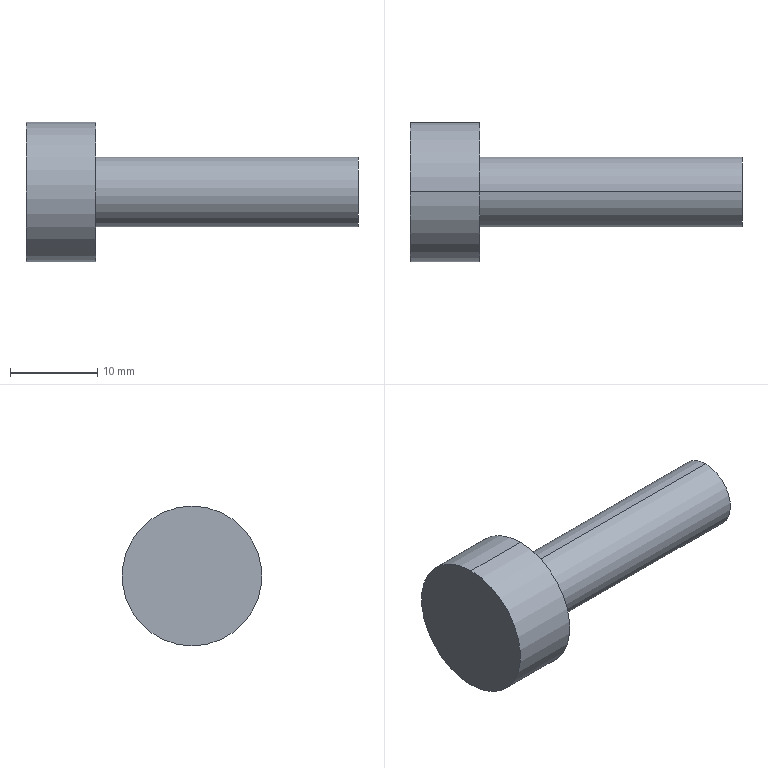Part | STEP file | 1 solid | 7 faces | box 38 x 16 x 16 mm | volume 3116 mm3 | cylinder 4 | plane 3 | commonest cylinder face diameters 8 x2 16 x2
STEP:
#1=CARTESIAN_POINT('',(0.,0.,0.));
#2=DIRECTION('',(0.,0.,1.));
#3=DIRECTION('',(1.,0.,0.));
#4=AXIS2_PLACEMENT_3D('',#1,#2,#3);
#5=CARTESIAN_POINT('',(-38.,0.,-8.));
#6=VERTEX_POINT('',#5);
#7=CARTESIAN_POINT('',(-38.,0.,8.));
#8=VERTEX_POINT('',#7);
#9=CARTESIAN_POINT('',(-38.,0.,0.));
#10=DIRECTION('',(1.,0.,0.));
#11=DIRECTION('',(0.,0.,-1.));
#12=AXIS2_PLACEMENT_3D('',#9,#10,#11);
#13=CIRCLE('',#12,8.);
#14=CARTESIAN_POINT('',(0.,0.,0.));
#15=DIRECTION('',(1.,0.,0.));
#16=DIRECTION('',(0.,0.,-1.));
#17=AXIS2_PLACEMENT_3D('',#14,#15,#16);
#18=CYLINDRICAL_SURFACE('',#17,8.);
#19=CARTESIAN_POINT('',(0.,-38.));
#20=DIRECTION('',(1.,0.));
#21=VECTOR('',#20,1.);
#22=LINE('',#19,#21);
#23=(GEOMETRIC_REPRESENTATION_CONTEXT(2)PARAMETRIC_REPRESENTATION_CONTEXT()REPRESENTATION_CONTEXT('',''));
#24=DEFINITIONAL_REPRESENTATION('',(#22),#23);
#25=PCURVE('',#18,#24);
#26=CARTESIAN_POINT('',(-38.,8.,0.));
#27=DIRECTION('',(-1.,0.,0.));
#28=DIRECTION('',(0.,0.,1.));
#29=AXIS2_PLACEMENT_3D('',#26,#27,#28);
#30=PLANE('',#29);
#31=CARTESIAN_POINT('',(-8.,-8.));
#32=CARTESIAN_POINT('',(-8.,5.856));
#33=CARTESIAN_POINT('',(4.,-1.072));
#34=CARTESIAN_POINT('',(16.,-8.));
#35=CARTESIAN_POINT('',(4.,-14.928));
#36=CARTESIAN_POINT('',(-8.,-21.856));
#37=CARTESIAN_POINT('',(-8.,-8.));
#38=(BOUNDED_CURVE()B_SPLINE_CURVE(2,(#31,#32,#33,#34,#35,#36,#37),.UNSPECIFIED.,.T.,.F.)B_SPLINE_CURVE_WITH_KNOTS((1,2,2,2,2,1),(-2.094,0.,2.094,4.189,6.283,8.378),.UNSPECIFIED.)CURVE()GEOMETRIC_REPRESENTATION_ITEM()RATIONAL_B_SPLINE_CURVE((1.,0.5,1.,0.5,1.,0.5,1.))REPRESENTATION_ITEM(''));
#39=(GEOMETRIC_REPRESENTATION_CONTEXT(2)PARAMETRIC_REPRESENTATION_CONTEXT()REPRESENTATION_CONTEXT('',''));
#40=DEFINITIONAL_REPRESENTATION('',(#38),#39);
#41=PCURVE('',#30,#40);
#42=SURFACE_CURVE('',#13,(#25,#41),.PCURVE_S1.);
#43=EDGE_CURVE('',#6,#8,#42,.T.);
#44=ORIENTED_EDGE('',*,*,#43,.T.);
#45=CARTESIAN_POINT('',(-30.,0.,8.));
#46=VERTEX_POINT('',#45);
#47=CARTESIAN_POINT('',(0.,0.,8.));
#48=DIRECTION('',(1.,0.,0.));
#49=VECTOR('',#48,1.);
#50=LINE('',#47,#49);
#51=CARTESIAN_POINT('',(3.142,0.));
#52=DIRECTION('',(0.,1.));
#53=VECTOR('',#52,1.);
#54=LINE('',#51,#53);
#55=(GEOMETRIC_REPRESENTATION_CONTEXT(2)PARAMETRIC_REPRESENTATION_CONTEXT()REPRESENTATION_CONTEXT('',''));
#56=DEFINITIONAL_REPRESENTATION('',(#54),#55);
#57=PCURVE('',#18,#56);
#58=CARTESIAN_POINT('',(0.,0.,0.));
#59=DIRECTION('',(1.,0.,0.));
#60=DIRECTION('',(0.,0.,-1.));
#61=AXIS2_PLACEMENT_3D('',#58,#59,#60);
#62=CYLINDRICAL_SURFACE('',#61,8.);
#63=CARTESIAN_POINT('',(3.142,0.));
#64=DIRECTION('',(0.,1.));
#65=VECTOR('',#64,1.);
#66=LINE('',#63,#65);
#67=(GEOMETRIC_REPRESENTATION_CONTEXT(2)PARAMETRIC_REPRESENTATION_CONTEXT()REPRESENTATION_CONTEXT('',''));
#68=DEFINITIONAL_REPRESENTATION('',(#66),#67);
#69=PCURVE('',#62,#68);
#70=SURFACE_CURVE('',#50,(#57,#69),.PCURVE_S1.);
#71=EDGE_CURVE('',#8,#46,#70,.T.);
#72=ORIENTED_EDGE('',*,*,#71,.T.);
#73=CARTESIAN_POINT('',(-30.,0.,-8.));
#74=VERTEX_POINT('',#73);
#75=CARTESIAN_POINT('',(-30.,0.,0.));
#76=DIRECTION('',(1.,0.,0.));
#77=DIRECTION('',(0.,0.,-1.));
#78=AXIS2_PLACEMENT_3D('',#75,#76,#77);
#79=CIRCLE('',#78,8.);
#80=CARTESIAN_POINT('',(0.,-30.));
#81=DIRECTION('',(1.,0.));
#82=VECTOR('',#81,1.);
#83=LINE('',#80,#82);
#84=(GEOMETRIC_REPRESENTATION_CONTEXT(2)PARAMETRIC_REPRESENTATION_CONTEXT()REPRESENTATION_CONTEXT('',''));
#85=DEFINITIONAL_REPRESENTATION('',(#83),#84);
#86=PCURVE('',#18,#85);
#87=CARTESIAN_POINT('',(-30.,4.,0.));
#88=DIRECTION('',(1.,0.,0.));
#89=DIRECTION('',(0.,0.,-1.));
#90=AXIS2_PLACEMENT_3D('',#87,#88,#89);
#91=PLANE('',#90);
#92=CARTESIAN_POINT('',(0.,-4.));
#93=DIRECTION('',(1.,0.));
#94=AXIS2_PLACEMENT_2D('',#92,#93);
#95=CIRCLE('',#94,8.);
#96=(GEOMETRIC_REPRESENTATION_CONTEXT(2)PARAMETRIC_REPRESENTATION_CONTEXT()REPRESENTATION_CONTEXT('',''));
#97=DEFINITIONAL_REPRESENTATION('',(#95),#96);
#98=PCURVE('',#91,#97);
#99=SURFACE_CURVE('',#79,(#86,#98),.PCURVE_S1.);
#100=EDGE_CURVE('',#74,#46,#99,.T.);
#101=ORIENTED_EDGE('',*,*,#100,.F.);
#102=CARTESIAN_POINT('',(0.,0.,-8.));
#103=DIRECTION('',(1.,0.,0.));
#104=VECTOR('',#103,1.);
#105=LINE('',#102,#104);
#106=CARTESIAN_POINT('',(0.,0.));
#107=DIRECTION('',(0.,1.));
#108=VECTOR('',#107,1.);
#109=LINE('',#106,#108);
#110=(GEOMETRIC_REPRESENTATION_CONTEXT(2)PARAMETRIC_REPRESENTATION_CONTEXT()REPRESENTATION_CONTEXT('',''));
#111=DEFINITIONAL_REPRESENTATION('',(#109),#110);
#112=PCURVE('',#18,#111);
#113=CARTESIAN_POINT('',(6.283,0.));
#114=DIRECTION('',(0.,1.));
#115=VECTOR('',#114,1.);
#116=LINE('',#113,#115);
#117=(GEOMETRIC_REPRESENTATION_CONTEXT(2)PARAMETRIC_REPRESENTATION_CONTEXT()REPRESENTATION_CONTEXT('',''));
#118=DEFINITIONAL_REPRESENTATION('',(#116),#117);
#119=PCURVE('',#62,#118);
#120=SURFACE_CURVE('',#105,(#112,#119),.PCURVE_S1.);
#121=EDGE_CURVE('',#6,#74,#120,.T.);
#122=ORIENTED_EDGE('',*,*,#121,.F.);
#123=EDGE_LOOP('',(#44,#72,#101,#122));
#124=FACE_BOUND('',#123,.T.);
#125=ADVANCED_FACE('',(#124),#18,.T.);
#126=CARTESIAN_POINT('',(-30.,0.,-4.));
#127=VERTEX_POINT('',#126);
#128=CARTESIAN_POINT('',(-30.,0.,4.));
#129=VERTEX_POINT('',#128);
#130=CARTESIAN_POINT('',(-30.,0.,0.));
#131=DIRECTION('',(1.,0.,0.));
#132=DIRECTION('',(0.,0.,-1.));
#133=AXIS2_PLACEMENT_3D('',#130,#131,#132);
#134=CIRCLE('',#133,4.);
#135=CARTESIAN_POINT('',(0.,0.,0.));
#136=DIRECTION('',(1.,0.,0.));
#137=DIRECTION('',(0.,0.,-1.));
#138=AXIS2_PLACEMENT_3D('',#135,#136,#137);
#139=CYLINDRICAL_SURFACE('',#138,4.);
#140=CARTESIAN_POINT('',(0.,-30.));
#141=DIRECTION('',(1.,0.));
#142=VECTOR('',#141,1.);
#143=LINE('',#140,#142);
#144=(GEOMETRIC_REPRESENTATION_CONTEXT(2)PARAMETRIC_REPRESENTATION_CONTEXT()REPRESENTATION_CONTEXT('',''));
#145=DEFINITIONAL_REPRESENTATION('',(#143),#144);
#146=PCURVE('',#139,#145);
#147=CARTESIAN_POINT('',(0.,-4.));
#148=DIRECTION('',(1.,0.));
#149=AXIS2_PLACEMENT_2D('',#147,#148);
#150=CIRCLE('',#149,4.);
#151=(GEOMETRIC_REPRESENTATION_CONTEXT(2)PARAMETRIC_REPRESENTATION_CONTEXT()REPRESENTATION_CONTEXT('',''));
#152=DEFINITIONAL_REPRESENTATION('',(#150),#151);
#153=PCURVE('',#91,#152);
#154=SURFACE_CURVE('',#134,(#146,#153),.PCURVE_S1.);
#155=EDGE_CURVE('',#127,#129,#154,.T.);
#156=ORIENTED_EDGE('',*,*,#155,.T.);
#157=CARTESIAN_POINT('',(0.,0.,4.));
#158=VERTEX_POINT('',#157);
#159=CARTESIAN_POINT('',(0.,0.,4.));
#160=DIRECTION('',(1.,0.,0.));
#161=VECTOR('',#160,1.);
#162=LINE('',#159,#161);
#163=CARTESIAN_POINT('',(3.142,0.));
#164=DIRECTION('',(0.,1.));
#165=VECTOR('',#164,1.);
#166=LINE('',#163,#165);
#167=(GEOMETRIC_REPRESENTATION_CONTEXT(2)PARAMETRIC_REPRESENTATION_CONTEXT()REPRESENTATION_CONTEXT('',''));
#168=DEFINITIONAL_REPRESENTATION('',(#166),#167);
#169=PCURVE('',#139,#168);
#170=CARTESIAN_POINT('',(0.,0.,0.));
#171=DIRECTION('',(1.,0.,0.));
#172=DIRECTION('',(0.,0.,-1.));
#173=AXIS2_PLACEMENT_3D('',#170,#171,#172);
#174=CYLINDRICAL_SURFACE('',#173,4.);
#175=CARTESIAN_POINT('',(3.142,0.));
#176=DIRECTION('',(0.,1.));
#177=VECTOR('',#176,1.);
#178=LINE('',#175,#177);
#179=(GEOMETRIC_REPRESENTATION_CONTEXT(2)PARAMETRIC_REPRESENTATION_CONTEXT()REPRESENTATION_CONTEXT('',''));
#180=DEFINITIONAL_REPRESENTATION('',(#178),#179);
#181=PCURVE('',#174,#180);
#182=SURFACE_CURVE('',#162,(#169,#181),.PCURVE_S1.);
#183=EDGE_CURVE('',#129,#158,#182,.T.);
#184=ORIENTED_EDGE('',*,*,#183,.T.);
#185=CARTESIAN_POINT('',(0.,0.,-4.));
#186=VERTEX_POINT('',#185);
#187=CARTESIAN_POINT('',(0.,0.,0.));
#188=DIRECTION('',(1.,0.,0.));
#189=DIRECTION('',(0.,0.,-1.));
#190=AXIS2_PLACEMENT_3D('',#187,#188,#189);
#191=CIRCLE('',#190,4.);
#192=CARTESIAN_POINT('',(0.,0.));
#193=DIRECTION('',(1.,0.));
#194=VECTOR('',#193,1.);
#195=LINE('',#192,#194);
#196=(GEOMETRIC_REPRESENTATION_CONTEXT(2)PARAMETRIC_REPRESENTATION_CONTEXT()REPRESENTATION_CONTEXT('',''));
#197=DEFINITIONAL_REPRESENTATION('',(#195),#196);
#198=PCURVE('',#139,#197);
#199=CARTESIAN_POINT('',(0.,0.,0.));
#200=DIRECTION('',(1.,0.,0.));
#201=DIRECTION('',(0.,0.,-1.));
#202=AXIS2_PLACEMENT_3D('',#199,#200,#201);
#203=PLANE('',#202);
#204=CARTESIAN_POINT('',(0.,0.));
#205=DIRECTION('',(1.,0.));
#206=AXIS2_PLACEMENT_2D('',#204,#205);
#207=CIRCLE('',#206,4.);
#208=(GEOMETRIC_REPRESENTATION_CONTEXT(2)PARAMETRIC_REPRESENTATION_CONTEXT()REPRESENTATION_CONTEXT('',''));
#209=DEFINITIONAL_REPRESENTATION('',(#207),#208);
#210=PCURVE('',#203,#209);
#211=SURFACE_CURVE('',#191,(#198,#210),.PCURVE_S1.);
#212=EDGE_CURVE('',#186,#158,#211,.T.);
#213=ORIENTED_EDGE('',*,*,#212,.F.);
#214=CARTESIAN_POINT('',(0.,0.,-4.));
#215=DIRECTION('',(1.,0.,0.));
#216=VECTOR('',#215,1.);
#217=LINE('',#214,#216);
#218=CARTESIAN_POINT('',(0.,0.));
#219=DIRECTION('',(0.,1.));
#220=VECTOR('',#219,1.);
#221=LINE('',#218,#220);
#222=(GEOMETRIC_REPRESENTATION_CONTEXT(2)PARAMETRIC_REPRESENTATION_CONTEXT()REPRESENTATION_CONTEXT('',''));
#223=DEFINITIONAL_REPRESENTATION('',(#221),#222);
#224=PCURVE('',#139,#223);
#225=CARTESIAN_POINT('',(6.283,0.));
#226=DIRECTION('',(0.,1.));
#227=VECTOR('',#226,1.);
#228=LINE('',#225,#227);
#229=(GEOMETRIC_REPRESENTATION_CONTEXT(2)PARAMETRIC_REPRESENTATION_CONTEXT()REPRESENTATION_CONTEXT('',''));
#230=DEFINITIONAL_REPRESENTATION('',(#228),#229);
#231=PCURVE('',#174,#230);
#232=SURFACE_CURVE('',#217,(#224,#231),.PCURVE_S1.);
#233=EDGE_CURVE('',#127,#186,#232,.T.);
#234=ORIENTED_EDGE('',*,*,#233,.F.);
#235=EDGE_LOOP('',(#156,#184,#213,#234));
#236=FACE_BOUND('',#235,.T.);
#237=ADVANCED_FACE('',(#236),#139,.T.);
#238=ORIENTED_EDGE('',*,*,#212,.T.);
#239=CARTESIAN_POINT('',(0.,0.,0.));
#240=DIRECTION('',(1.,0.,0.));
#241=DIRECTION('',(0.,0.,-1.));
#242=AXIS2_PLACEMENT_3D('',#239,#240,#241);
#243=CIRCLE('',#242,4.);
#244=CARTESIAN_POINT('',(0.,0.));
#245=DIRECTION('',(1.,0.));
#246=AXIS2_PLACEMENT_2D('',#244,#245);
#247=CIRCLE('',#246,4.);
#248=(GEOMETRIC_REPRESENTATION_CONTEXT(2)PARAMETRIC_REPRESENTATION_CONTEXT()REPRESENTATION_CONTEXT('',''));
#249=DEFINITIONAL_REPRESENTATION('',(#247),#248);
#250=PCURVE('',#203,#249);
#251=CARTESIAN_POINT('',(0.,0.));
#252=DIRECTION('',(1.,0.));
#253=VECTOR('',#252,1.);
#254=LINE('',#251,#253);
#255=(GEOMETRIC_REPRESENTATION_CONTEXT(2)PARAMETRIC_REPRESENTATION_CONTEXT()REPRESENTATION_CONTEXT('',''));
#256=DEFINITIONAL_REPRESENTATION('',(#254),#255);
#257=PCURVE('',#174,#256);
#258=SURFACE_CURVE('',#243,(#250,#257),.PCURVE_S1.);
#259=EDGE_CURVE('',#158,#186,#258,.T.);
#260=ORIENTED_EDGE('',*,*,#259,.T.);
#261=EDGE_LOOP('',(#238,#260));
#262=FACE_BOUND('',#261,.T.);
#263=ADVANCED_FACE('',(#262),#203,.T.);
#264=ORIENTED_EDGE('',*,*,#183,.F.);
#265=CARTESIAN_POINT('',(-30.,0.,0.));
#266=DIRECTION('',(1.,0.,0.));
#267=DIRECTION('',(0.,0.,-1.));
#268=AXIS2_PLACEMENT_3D('',#265,#266,#267);
#269=CIRCLE('',#268,4.);
#270=CARTESIAN_POINT('',(0.,-30.));
#271=DIRECTION('',(1.,0.));
#272=VECTOR('',#271,1.);
#273=LINE('',#270,#272);
#274=(GEOMETRIC_REPRESENTATION_CONTEXT(2)PARAMETRIC_REPRESENTATION_CONTEXT()REPRESENTATION_CONTEXT('',''));
#275=DEFINITIONAL_REPRESENTATION('',(#273),#274);
#276=PCURVE('',#174,#275);
#277=CARTESIAN_POINT('',(0.,-4.));
#278=DIRECTION('',(1.,0.));
#279=AXIS2_PLACEMENT_2D('',#277,#278);
#280=CIRCLE('',#279,4.);
#281=(GEOMETRIC_REPRESENTATION_CONTEXT(2)PARAMETRIC_REPRESENTATION_CONTEXT()REPRESENTATION_CONTEXT('',''));
#282=DEFINITIONAL_REPRESENTATION('',(#280),#281);
#283=PCURVE('',#91,#282);
#284=SURFACE_CURVE('',#269,(#276,#283),.PCURVE_S1.);
#285=EDGE_CURVE('',#129,#127,#284,.T.);
#286=ORIENTED_EDGE('',*,*,#285,.T.);
#287=ORIENTED_EDGE('',*,*,#233,.T.);
#288=ORIENTED_EDGE('',*,*,#259,.F.);
#289=EDGE_LOOP('',(#264,#286,#287,#288));
#290=FACE_BOUND('',#289,.T.);
#291=ADVANCED_FACE('',(#290),#174,.T.);
#292=ORIENTED_EDGE('',*,*,#100,.T.);
#293=CARTESIAN_POINT('',(-30.,0.,0.));
#294=DIRECTION('',(1.,0.,0.));
#295=DIRECTION('',(0.,0.,-1.));
#296=AXIS2_PLACEMENT_3D('',#293,#294,#295);
#297=CIRCLE('',#296,8.);
#298=CARTESIAN_POINT('',(0.,-4.));
#299=DIRECTION('',(1.,0.));
#300=AXIS2_PLACEMENT_2D('',#298,#299);
#301=CIRCLE('',#300,8.);
#302=(GEOMETRIC_REPRESENTATION_CONTEXT(2)PARAMETRIC_REPRESENTATION_CONTEXT()REPRESENTATION_CONTEXT('',''));
#303=DEFINITIONAL_REPRESENTATION('',(#301),#302);
#304=PCURVE('',#91,#303);
#305=CARTESIAN_POINT('',(0.,-30.));
#306=DIRECTION('',(1.,0.));
#307=VECTOR('',#306,1.);
#308=LINE('',#305,#307);
#309=(GEOMETRIC_REPRESENTATION_CONTEXT(2)PARAMETRIC_REPRESENTATION_CONTEXT()REPRESENTATION_CONTEXT('',''));
#310=DEFINITIONAL_REPRESENTATION('',(#308),#309);
#311=PCURVE('',#62,#310);
#312=SURFACE_CURVE('',#297,(#304,#311),.PCURVE_S1.);
#313=EDGE_CURVE('',#46,#74,#312,.T.);
#314=ORIENTED_EDGE('',*,*,#313,.T.);
#315=EDGE_LOOP('',(#292,#314));
#316=FACE_BOUND('',#315,.T.);
#317=ORIENTED_EDGE('',*,*,#155,.F.);
#318=ORIENTED_EDGE('',*,*,#285,.F.);
#319=EDGE_LOOP('',(#317,#318));
#320=FACE_BOUND('',#319,.T.);
#321=ADVANCED_FACE('',(#316,#320),#91,.T.);
#322=ORIENTED_EDGE('',*,*,#71,.F.);
#323=CARTESIAN_POINT('',(-38.,0.,0.));
#324=DIRECTION('',(1.,0.,0.));
#325=DIRECTION('',(0.,0.,-1.));
#326=AXIS2_PLACEMENT_3D('',#323,#324,#325);
#327=CIRCLE('',#326,8.);
#328=CARTESIAN_POINT('',(0.,-38.));
#329=DIRECTION('',(1.,0.));
#330=VECTOR('',#329,1.);
#331=LINE('',#328,#330);
#332=(GEOMETRIC_REPRESENTATION_CONTEXT(2)PARAMETRIC_REPRESENTATION_CONTEXT()REPRESENTATION_CONTEXT('',''));
#333=DEFINITIONAL_REPRESENTATION('',(#331),#332);
#334=PCURVE('',#62,#333);
#335=CARTESIAN_POINT('',(-8.,-8.));
#336=CARTESIAN_POINT('',(-8.,5.856));
#337=CARTESIAN_POINT('',(4.,-1.072));
#338=CARTESIAN_POINT('',(16.,-8.));
#339=CARTESIAN_POINT('',(4.,-14.928));
#340=CARTESIAN_POINT('',(-8.,-21.856));
#341=CARTESIAN_POINT('',(-8.,-8.));
#342=(BOUNDED_CURVE()B_SPLINE_CURVE(2,(#335,#336,#337,#338,#339,#340,#341),.UNSPECIFIED.,.T.,.F.)B_SPLINE_CURVE_WITH_KNOTS((1,2,2,2,2,1),(-2.094,0.,2.094,4.189,6.283,8.378),.UNSPECIFIED.)CURVE()GEOMETRIC_REPRESENTATION_ITEM()RATIONAL_B_SPLINE_CURVE((1.,0.5,1.,0.5,1.,0.5,1.))REPRESENTATION_ITEM(''));
#343=(GEOMETRIC_REPRESENTATION_CONTEXT(2)PARAMETRIC_REPRESENTATION_CONTEXT()REPRESENTATION_CONTEXT('',''));
#344=DEFINITIONAL_REPRESENTATION('',(#342),#343);
#345=PCURVE('',#30,#344);
#346=SURFACE_CURVE('',#327,(#334,#345),.PCURVE_S1.);
#347=EDGE_CURVE('',#8,#6,#346,.T.);
#348=ORIENTED_EDGE('',*,*,#347,.T.);
#349=ORIENTED_EDGE('',*,*,#121,.T.);
#350=ORIENTED_EDGE('',*,*,#313,.F.);
#351=EDGE_LOOP('',(#322,#348,#349,#350));
#352=FACE_BOUND('',#351,.T.);
#353=ADVANCED_FACE('',(#352),#62,.T.);
#354=ORIENTED_EDGE('',*,*,#43,.F.);
#355=ORIENTED_EDGE('',*,*,#347,.F.);
#356=EDGE_LOOP('',(#354,#355));
#357=FACE_BOUND('',#356,.T.);
#358=ADVANCED_FACE('',(#357),#30,.T.);
#359=CLOSED_SHELL('',(#125,#237,#263,#291,#321,#353,#358));
#360=MANIFOLD_SOLID_BREP('',#359);
#361=(LENGTH_UNIT()NAMED_UNIT(*)SI_UNIT(.MILLI.,.METRE.));
#362=UNCERTAINTY_MEASURE_WITH_UNIT(LENGTH_MEASURE(0.0000001),#361,'','');
#363=(NAMED_UNIT(*)PLANE_ANGLE_UNIT()SI_UNIT($,.RADIAN.));
#364=(NAMED_UNIT(*)SI_UNIT($,.STERADIAN.)SOLID_ANGLE_UNIT());
#365=(GEOMETRIC_REPRESENTATION_CONTEXT(3)GLOBAL_UNCERTAINTY_ASSIGNED_CONTEXT((#362))GLOBAL_UNIT_ASSIGNED_CONTEXT((#361,#363,#364))REPRESENTATION_CONTEXT('',''));
#366=ADVANCED_BREP_SHAPE_REPRESENTATION('',(#4,#360),#365);